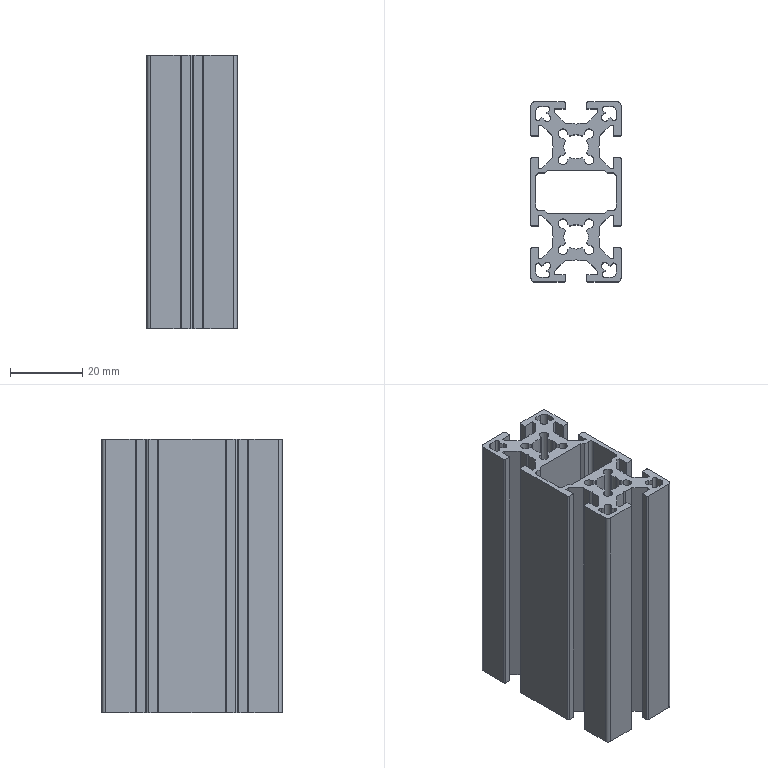Part | STEP file | HFS5-2550-300 | 1 solid | 230 faces | box 25 x 50.001 x 76 mm | volume 38256 mm3 | plane 136 | cylinder 94 | commonest cylinder face diameters 0.6 x30 2.6 x24 2 x13 1.4 x10 6.8 x10 3 x4